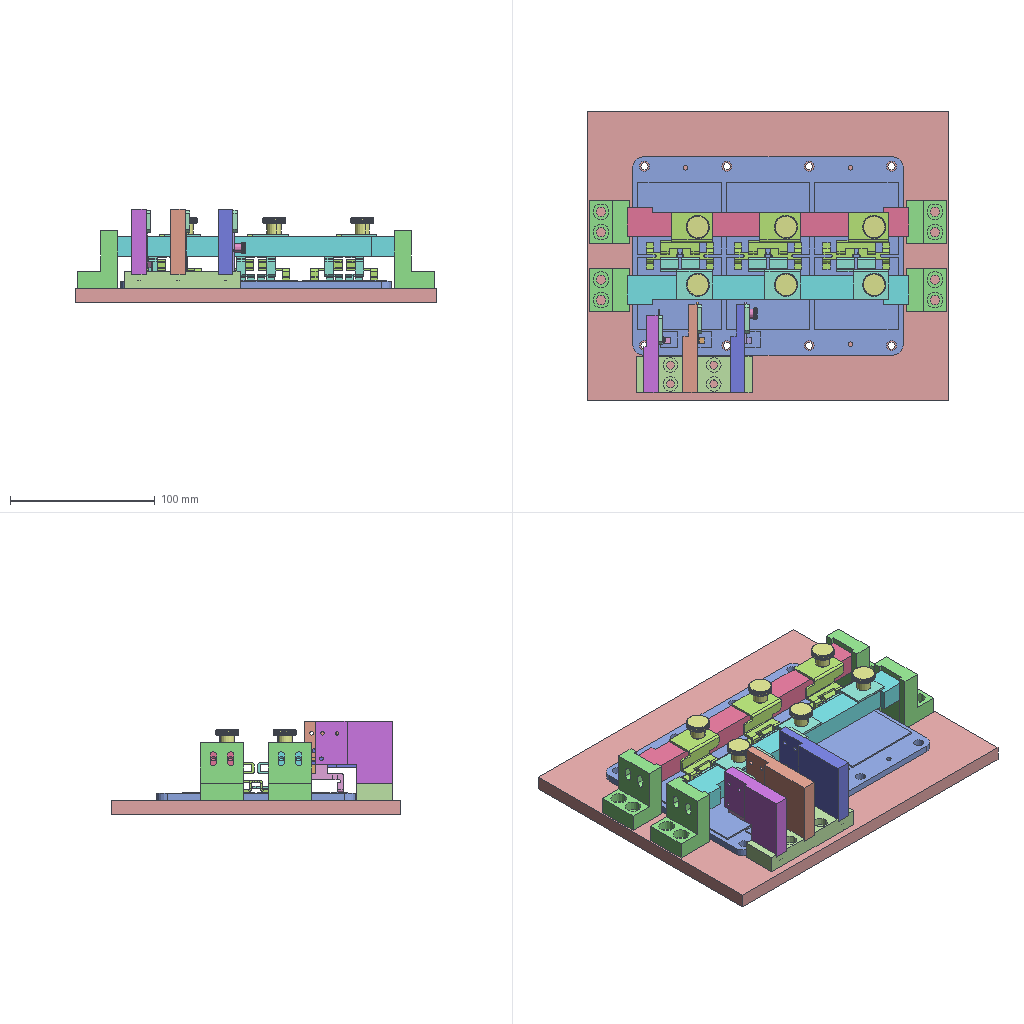Assembly | SolidWorks | 22 different items | 43 placed | box 250 x 200 x 65 mm
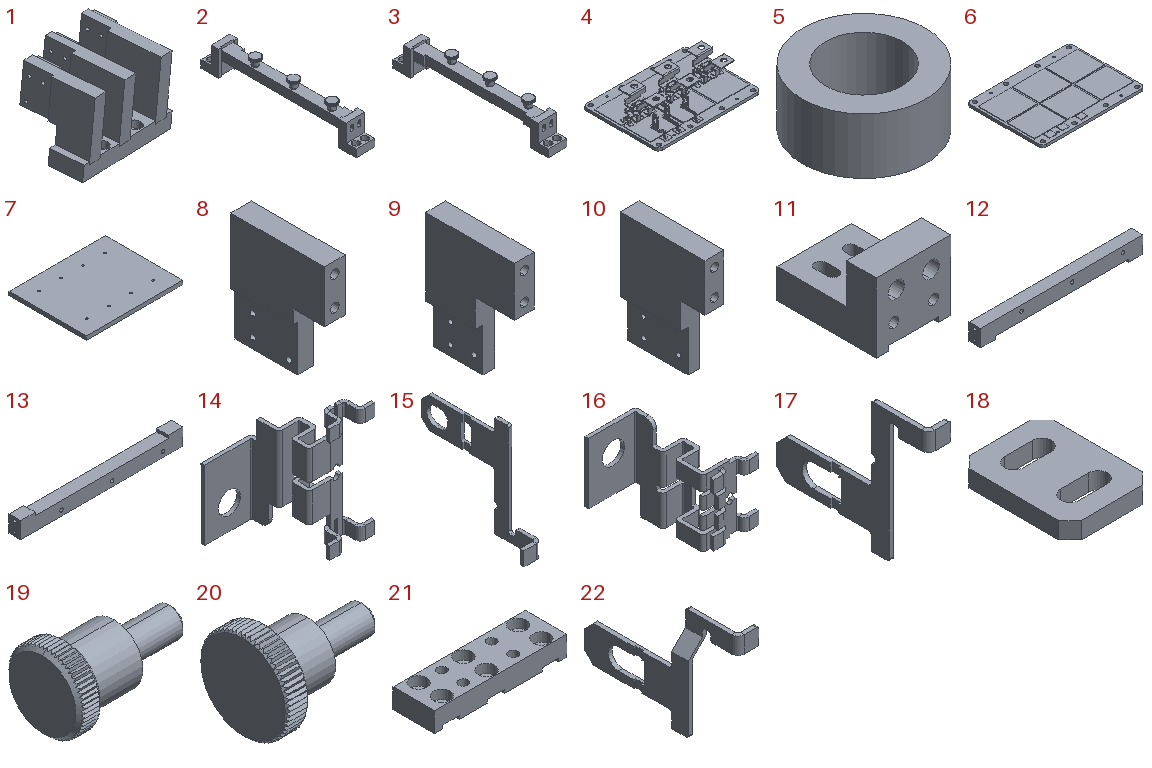Parts list (item | name | quantity | parent item | size | volume | features):
1 | (subassembly) | x1 | - | 82.95 x 68.99 x 62.182 mm | 75184 mm3 | -
2 | (subassembly) | x1 | - | 30 x 247 x 49 mm | 82433 mm3 | features ReferencePattern 4, LocalLPattern 1
3 | (subassembly) | x1 | - | 30 x 247 x 49 mm | 82433 mm3 | features ReferencePattern 4, LocalLPattern 1
4 | (subassembly) | x1 | - | 187 x 137 x 38.97 mm | 158216 mm3 | features ReferencePattern 4, LocalLPattern 1
5 | - | x6 | in 2, 3 | 8.8 x 8.8 x 4 mm | 148.252 mm3 | features Extrusion 1
6 | - | x1 | in 4 | 187 x 137 x 5.87 mm | 140466 mm3 | features ICE 3, HoleWzd 2, Extrusion 1, Fillet 1
7 | - | x1 | - | 250 x 200 x 10 mm | 498429 mm3 | features Extrusion 1, HoleWzd 1
8 | - | x1 | in 1 | 10.8 x 45 x 53.5 mm | 18015 mm3 | features ICE 4, HoleWzd 3, ExtruThin 1
9 | - | x1 | in 1 | 10.8 x 45 x 61 mm | 17616 mm3 | features ICE 4, HoleWzd 3, ExtruThin 1, Fillet 1
10 | - | x1 | in 1 | 10.8 x 45 x 61 mm | 19522 mm3 | features ICE 4, HoleWzd 3, ExtruThin 1
11 | - | x4 | in 2, 3 | 30 x 40 x 28 mm | 15981 mm3 | features HoleWzd 4, ICE 3, Extrusion 1
12 | - | x1 | in 2 | 195 x 14 x 20 mm | 45399 mm3 | features HoleWzd 3, ICE 2, ExtruThin 1
13 | - | x1 | in 3 | 195 x 14 x 20 mm | 45399 mm3 | features HoleWzd 3, ICE 2, ExtruThin 1
14 | - | x3 | in 4 | 39.2 x 31.5 x 46.3 mm | 2979 mm3 | features ICE 8, Fillet 4, FlatPattern 1, SMBaseFlange 1, SheetMetal 1
15 | - | x1 | in 4 | 5 x 33.1 x 28.5 mm | 287.645 mm3 | features ICE 7, Chamfer 1, EdgeFlange 1, Fillet 1, FlatPattern 1, SMBaseFlange 1, SheetMetal 1
16 | - | x3 | in 4 | 39.2 x 31.5 x 36.05 mm | 2657 mm3 | features ICE 10, Fillet 4, FlatPattern 1, LPattern 1, SMBaseFlange 1, SheetMetal 1
17 | - | x1 | in 4 | 5 x 33.1 x 28.5 mm | 286.856 mm3 | features ICE 6, FlatPattern 2, Chamfer 1, Fillet 1, MirrorSolid 1, SMBaseFlange 1, SheetMetal 1
18 | - | x3 | in 1 | 15 x 20 x 3 mm | 719.525 mm3 | features Chamfer 1, Extrusion 1, HoleWzd 1
19 | - | x3 | in 1 | 13.5 x 8 x 8 mm | 298.871 mm3 | features MBimport 1
20 | - | x6 | in 2, 3 | 21.5 x 16 x 16 mm | 1542 mm3 | features MBimport 1
21 | - | x1 | in 1 | 80 x 25 x 12 mm | 16976 mm3 | features HoleWzd 2, Extrusion 1, ICE 1
22 | - | x1 | in 4 | 8.33 x 33.1 x 23.2 mm | 267.226 mm3 | features ICE 5, Chamfer 1, Fillet 1, FlatPattern 1, SMBaseFlange 1, SheetMetal 1
Mates (type | each side: item.copy, entity, surface, feature):
In the top assembly
Coincident | 7.1 face plane Boss-Extrude1 | 6.1 face plane Boss-Extrude1
Concentric | 7.1 face cylinder M6 Tapped Hole1 | 6.1 face cylinder Ø7.0 (7) Diameter Hole1
Concentric | 7.1 edge | 6.1 face cylinder Ø7.0 (7) Diameter Hole1
Coincident | 7.1 face plane Boss-Extrude1 | 11.1 face plane Boss-Extrude1
Width | 11.1 face plane Boss-Extrude1 | 11.2 face plane Boss-Extrude1 | 6.1 face plane Boss-Extrude1 | 6.1 face plane Boss-Extrude1
DistanceDim | 11.1 face plane Boss-Extrude1 | 6.1 face plane Boss-Extrude1
Coincident | 7.1 face plane Boss-Extrude1 | 11.3 face plane Boss-Extrude1
Coincident | 11.1 face plane Boss-Extrude1 | 11.3 face plane Boss-Extrude1
DistanceDim | 11.3 face plane Boss-Extrude1 | 11.1 face plane Boss-Extrude1
Coincident | 7.1 face plane Boss-Extrude1 | 21.1 face plane Boss-Extrude1
DistanceDim | 21.1 face plane Boss-Extrude1 | 6.1 face plane Boss-Extrude1 | 2 times
In subassembly 2
Coincident | 11.4 face plane Cut-Extrude2 | 12.1 face plane Extrude-Thin1
Slot | 11.4 face plane M4 Clearance Slot2 | 12.1 face cylinder M4 Tapped Hole2 | 2 times
Coincident | 12.1 face plane Extrude-Thin1 | 11.5 face plane Cut-Extrude2
Coincident | 11.5 face plane Boss-Extrude1 | 11.4 face plane Boss-Extrude1
Coincident | 11.5 face plane Boss-Extrude2 | 11.4 face plane Boss-Extrude2
Concentric | 12.1 face cylinder Cut-Extrude1 | 5.1 face cylinder Boss-Extrude1
Coincident | 12.1 face plane Cut-Extrude1 | 5.1 face plane Boss-Extrude1
Concentric | 5.1 face cylinder Boss-Extrude1 | 20.1 face cylinder NKOSC5-10-16.stp<1>
DistanceDim | 12.1 face plane Extrude-Thin1 | 20.1 face plane NKOSC5-10-16.stp<1>
In subassembly 1
Concentric | 8.1 face cylinder M3 Tapped Hole1 | 19.1 face cylinder NKOSC3-6-8.stp<1>
DistanceDim | 8.1 face plane Extrude-Thin1 | 19.1 face plane NKOSC3-6-8.stp<1>
Coincident | 8.1 face plane Extrude-Thin1 | 18.1 face plane Boss-Extrude1
Slot | 18.1 face plane M3 Clearance Slot1 | 8.1 face cylinder M3 Tapped Hole2
Slot | 8.1 face cylinder M3 Tapped Hole2 | 18.1 face plane M3 Clearance Slot1
Parallel | 8.1 face plane Cut-Extrude2 | 21.2 face plane Cut-Extrude1
Coincident | 8.1 face plane Extrude-Thin1 | 21.2 face plane Boss-Extrude1
Coincident | 8.1 face plane Extrude-Thin1 | 21.2 face plane Cut-Extrude1
Coincident | 8.1 face plane Cut-Extrude2 | 21.2 face plane Cut-Extrude1
Coincident | 9.1 face plane Extrude-Thin1 | 18.2 face plane Boss-Extrude1
Slot | 18.2 face cylinder M3 Clearance Slot1 | 9.1 face cylinder M3 Tapped Hole1 | 2 times
Coincident | 9.1 face plane Cut-Extrude2 | 21.2 face plane Cut-Extrude1
Concentric | 9.1 face cylinder M3 Tapped Hole2 | 19.2 face cylinder NKOSC3-6-8.stp<1>
DistanceDim | 9.1 face plane Extrude-Thin1 | 19.2 face plane NKOSC3-6-8.stp<1>
DistanceDim | 9.1 face plane Extrude-Thin1 | 8.1 face plane Extrude-Thin1
Coincident | 8.1 face plane Extrude-Thin1 | 9.1 face plane Extrude-Thin1
Coincident | 10.1 face plane Extrude-Thin1 | 18.3 face plane Boss-Extrude1
Slot | 18.3 face cylinder M3 Clearance Slot1 | 10.1 face cylinder M3 Tapped Hole1 | 2 times
Coincident | 10.1 face plane Extrude-Thin1 | 21.2 face plane Cut-Extrude1
Concentric | 10.1 face cylinder M5 Tapped Hole1 | 21.2 face cylinder CBORE for M5 Hex Socket Head Cap Screw1
Coincident | 10.1 face plane Cut-Extrude2 | 21.2 face plane Cut-Extrude1
Concentric | 10.1 face cylinder M3 Tapped Hole2 | 19.3 face cylinder NKOSC3-6-8.stp<1>
DistanceDim | 10.1 face plane Extrude-Thin1 | 19.3 face plane NKOSC3-6-8.stp<1>
Coincident | 9.1 face plane Extrude-Thin1 | 10.1 face plane Extrude-Thin1
In subassembly 4
Coincident | 6.2 face plane Boss-Extrude3 | 22.1 face plane Base-Flange1
DistanceDim | 22.1 face plane Base-Flange1 | 6.2 face plane Boss-Extrude3 | 2 times
DistanceDim | 15.1 face plane Edge-Flange1 | 6.2 face plane Boss-Extrude3
Coincident | 6.2 face plane Boss-Extrude3 | 15.1 face plane Edge-Flange1
DistanceDim | 6.2 face plane Boss-Extrude3 | 15.1 face plane Edge-Flange1
Coincident | 6.2 face plane Boss-Extrude3 | 17.1 face plane Mirror2
DistanceDim | 17.1 face plane Mirror2 | 6.2 face plane Boss-Extrude3
DistanceDim | 17.1 face plane Mirror2 | 6.2 edge
Coincident | 6.2 face plane Boss-Extrude2 | 14.1 face plane Base-Flange1
Coincident | 6.2 face plane Boss-Extrude2 | 16.1 face plane Base-Flange1
DistanceDim | 16.1 face cylinder Cut-Extrude5 | 6.2 face plane Boss-Extrude2 | 2 times
Parallel | 6.2 face plane Boss-Extrude1 | 16.1 face plane Cut-Extrude4
DistanceDim | 14.1 face cylinder Cut-Extrude5 | 6.2 face plane Boss-Extrude2
DistanceDim | 6.2 face plane Boss-Extrude2 | 14.1 face cylinder Cut-Extrude5
Parallel | 6.2 face plane Boss-Extrude2 | 14.1 face plane Base-Flange1
In subassembly 3
Coincident | 11.4 face plane Cut-Extrude2 | 13.1 face plane Extrude-Thin1
Slot | 11.4 face plane M4 Clearance Slot2 | 13.1 face cylinder M4 Tapped Hole2 | 2 times
Coincident | 13.1 face plane Extrude-Thin1 | 11.5 face plane Cut-Extrude2
Coincident | 11.5 face plane Boss-Extrude1 | 11.4 face plane Boss-Extrude1
Coincident | 11.5 face plane Boss-Extrude2 | 11.4 face plane Boss-Extrude2
Concentric | 13.1 face cylinder Cut-Extrude1 | 5.1 face cylinder Boss-Extrude1
Coincident | 13.1 face plane Cut-Extrude1 | 5.1 face plane Boss-Extrude1
Concentric | 5.1 face cylinder Boss-Extrude1 | 20.1 face cylinder NKOSC5-10-16.stp<1>
DistanceDim | 13.1 face plane Extrude-Thin1 | 20.1 face plane NKOSC5-10-16.stp<1>